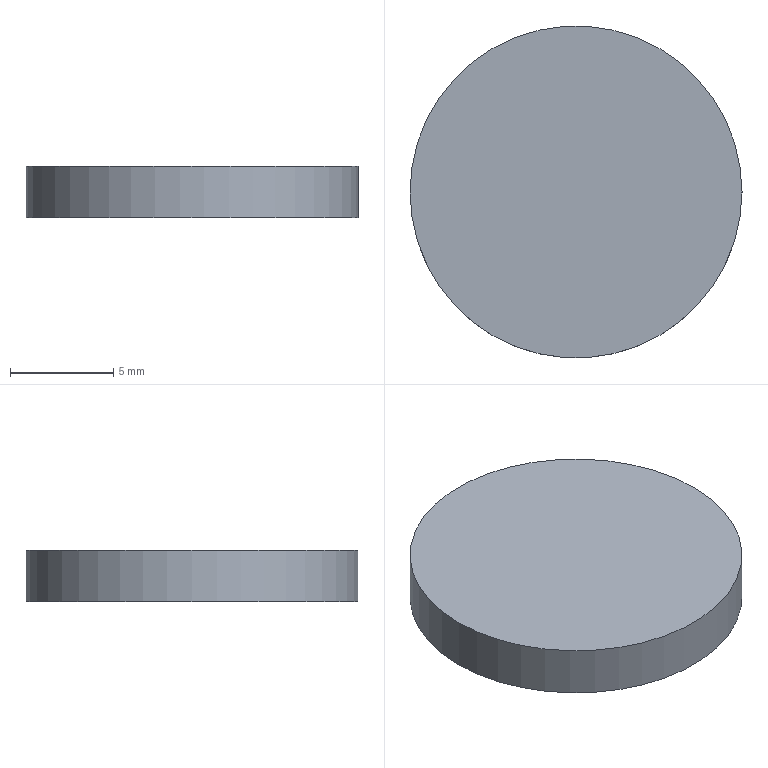Part | STEP file | lll_id1254_x_t | 1 solid | 3 faces | box 16.1 x 16.1 x 2.5 mm | volume 508.958 mm3 | plane 2 | cylinder 1 | commonest cylinder face diameters 16.1 x1
STEP:
#1=CARTESIAN_POINT('',(882.95,0.,2.5));
#2=VERTEX_POINT('',#1);
#3=CARTESIAN_POINT('',(891.,0.,2.5));
#4=DIRECTION('',(0.,0.,1.));
#5=DIRECTION('',(-1.,0.,0.));
#6=AXIS2_PLACEMENT_3D('',#3,#4,#5);
#7=CIRCLE('',#6,8.05);
#8=EDGE_CURVE('',#2,#2,#7,.T.);
#9=ORIENTED_EDGE('',*,*,#8,.F.);
#10=EDGE_LOOP('',(#9));
#11=FACE_BOUND('',#10,.T.);
#12=CARTESIAN_POINT('',(882.95,0.,0.));
#13=VERTEX_POINT('',#12);
#14=CARTESIAN_POINT('',(891.,0.,0.));
#15=DIRECTION('',(0.,0.,1.));
#16=DIRECTION('',(-1.,0.,0.));
#17=AXIS2_PLACEMENT_3D('',#14,#15,#16);
#18=CIRCLE('',#17,8.05);
#19=EDGE_CURVE('',#13,#13,#18,.T.);
#20=ORIENTED_EDGE('',*,*,#19,.T.);
#21=EDGE_LOOP('',(#20));
#22=FACE_BOUND('',#21,.T.);
#23=CARTESIAN_POINT('',(891.,0.,2.5));
#24=DIRECTION('',(0.,0.,-1.));
#25=DIRECTION('',(-1.,0.,0.));
#26=AXIS2_PLACEMENT_3D('',#23,#24,#25);
#27=CYLINDRICAL_SURFACE('',#26,8.05);
#28=ADVANCED_FACE('',(#11,#22),#27,.T.);
#29=ORIENTED_EDGE('',*,*,#8,.T.);
#30=EDGE_LOOP('',(#29));
#31=FACE_OUTER_BOUND('',#30,.T.);
#32=CARTESIAN_POINT('',(891.,0.,2.5));
#33=DIRECTION('',(0.,0.,1.));
#34=DIRECTION('',(1.,0.,0.));
#35=AXIS2_PLACEMENT_3D('',#32,#33,#34);
#36=PLANE('',#35);
#37=ADVANCED_FACE('',(#31),#36,.T.);
#38=ORIENTED_EDGE('',*,*,#19,.F.);
#39=EDGE_LOOP('',(#38));
#40=FACE_OUTER_BOUND('',#39,.T.);
#41=CARTESIAN_POINT('',(891.,0.,0.));
#42=DIRECTION('',(0.,0.,1.));
#43=DIRECTION('',(1.,0.,0.));
#44=AXIS2_PLACEMENT_3D('',#41,#42,#43);
#45=PLANE('',#44);
#46=ADVANCED_FACE('',(#40),#45,.F.);
#47=CLOSED_SHELL('',(#28,#37,#46));
#48=MANIFOLD_SOLID_BREP('',#47);
#49=(LENGTH_UNIT()NAMED_UNIT(*)SI_UNIT(.MILLI.,.METRE.));
#50=UNCERTAINTY_MEASURE_WITH_UNIT(LENGTH_MEASURE(0.00002),#49,'','');
#51=(NAMED_UNIT(*)PLANE_ANGLE_UNIT()SI_UNIT($,.RADIAN.));
#52=PLANE_ANGLE_MEASURE_WITH_UNIT(PLANE_ANGLE_MEASURE(0.01745),#51);
#53=DIMENSIONAL_EXPONENTS(0.,0.,0.,0.,0.,0.,0.);
#54=(CONVERSION_BASED_UNIT('DEGREE',#52)NAMED_UNIT(#53)PLANE_ANGLE_UNIT());
#55=(NAMED_UNIT(*)SI_UNIT($,.STERADIAN.)SOLID_ANGLE_UNIT());
#56=(GEOMETRIC_REPRESENTATION_CONTEXT(3)GLOBAL_UNCERTAINTY_ASSIGNED_CONTEXT((#50))GLOBAL_UNIT_ASSIGNED_CONTEXT((#49,#54,#55))REPRESENTATION_CONTEXT('',''));
#57=ADVANCED_BREP_SHAPE_REPRESENTATION('',(#48),#56);